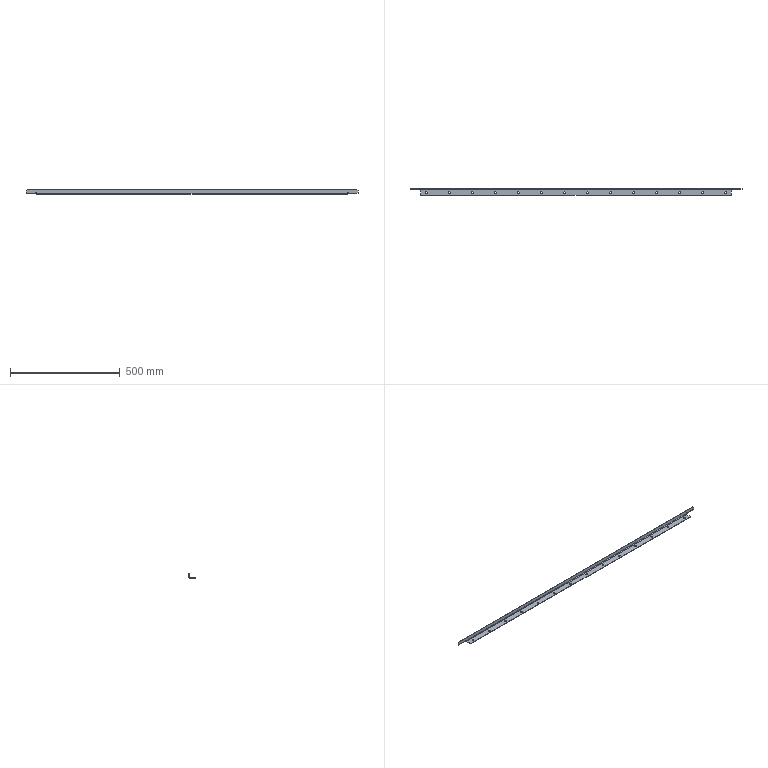Part | SolidWorks | features ICE 2, Chamfer 1, FlatPattern 1, SMBaseFlange 1, SheetMetal 1 | 1 solid | 61 faces | box 1515 x 30 x 20 mm | volume 133571 mm3 | cylinder 37 | plane 24 | commonest cylinder face diameters 8 x28 3 x3 5 x3 9 x3